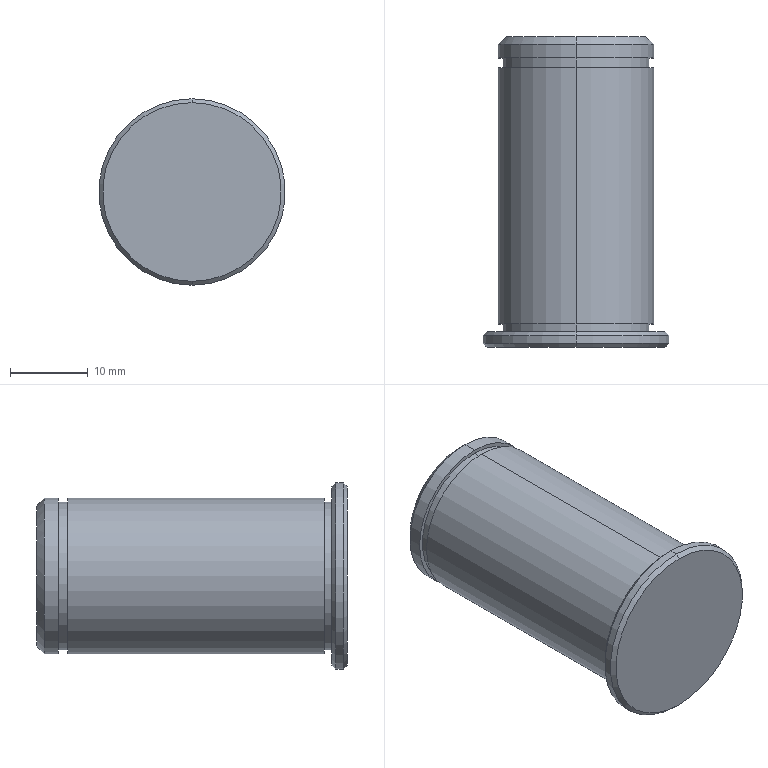Part | SolidWorks | features Revolution 1 | 1 solid | 22 faces | box 24 x 40 x 24 mm | volume 12725 mm3 | cylinder 10 | cone 6 | plane 6 | commonest cylinder face diameters 19 x4 20 x4 24 x2
STEP:
#1=CARTESIAN_POINT('',(0.,0.,-11.5));
#2=VERTEX_POINT('',#1);
#3=CARTESIAN_POINT('',(0.,0.,11.5));
#4=VERTEX_POINT('',#3);
#5=CARTESIAN_POINT('',(0.,0.,0.));
#6=DIRECTION('',(0.,-1.,0.));
#7=DIRECTION('',(0.,0.,-1.));
#8=AXIS2_PLACEMENT_3D('',#5,#6,#7);
#9=CIRCLE('',#8,11.5);
#10=EDGE_CURVE('',#2,#4,#9,.T.);
#11=ORIENTED_EDGE('',*,*,#10,.F.);
#12=CARTESIAN_POINT('',(0.,0.5,-12.));
#13=VERTEX_POINT('',#12);
#14=CARTESIAN_POINT('',(0.,0.,-11.5));
#15=DIRECTION('',(0.,0.7071,-0.7071));
#16=VECTOR('',#15,1000.);
#17=LINE('',#14,#16);
#18=EDGE_CURVE('',#2,#13,#17,.T.);
#19=ORIENTED_EDGE('',*,*,#18,.T.);
#20=CARTESIAN_POINT('',(0.,0.5,12.));
#21=VERTEX_POINT('',#20);
#22=CARTESIAN_POINT('',(0.,0.5,0.));
#23=DIRECTION('',(0.,-1.,0.));
#24=DIRECTION('',(0.,0.,-1.));
#25=AXIS2_PLACEMENT_3D('',#22,#23,#24);
#26=CIRCLE('',#25,12.);
#27=EDGE_CURVE('',#13,#21,#26,.T.);
#28=ORIENTED_EDGE('',*,*,#27,.T.);
#29=CARTESIAN_POINT('',(0.,0.,11.5));
#30=DIRECTION('',(0.,0.7071,0.7071));
#31=VECTOR('',#30,1000.);
#32=LINE('',#29,#31);
#33=EDGE_CURVE('',#4,#21,#32,.T.);
#34=ORIENTED_EDGE('',*,*,#33,.F.);
#35=EDGE_LOOP('',(#11,#19,#28,#34));
#36=FACE_OUTER_BOUND('',#35,.T.);
#37=CARTESIAN_POINT('',(0.,0.,0.));
#38=DIRECTION('',(0.,1.,0.));
#39=DIRECTION('',(0.,0.,1.));
#40=AXIS2_PLACEMENT_3D('',#37,#38,#39);
#41=CONICAL_SURFACE('',#40,11.5,0.7854);
#42=ADVANCED_FACE('',(#36),#41,.T.);
#43=CARTESIAN_POINT('',(0.,1.5,-12.));
#44=VERTEX_POINT('',#43);
#45=CARTESIAN_POINT('',(0.,1.5,12.));
#46=VERTEX_POINT('',#45);
#47=CARTESIAN_POINT('',(0.,1.5,0.));
#48=DIRECTION('',(0.,-1.,0.));
#49=DIRECTION('',(0.,0.,-1.));
#50=AXIS2_PLACEMENT_3D('',#47,#48,#49);
#51=CIRCLE('',#50,12.);
#52=EDGE_CURVE('',#44,#46,#51,.T.);
#53=ORIENTED_EDGE('',*,*,#52,.T.);
#54=CARTESIAN_POINT('',(0.,-1.467,12.));
#55=DIRECTION('',(0.,-1.,0.));
#56=VECTOR('',#55,1000.);
#57=LINE('',#54,#56);
#58=EDGE_CURVE('',#46,#21,#57,.T.);
#59=ORIENTED_EDGE('',*,*,#58,.T.);
#60=ORIENTED_EDGE('',*,*,#27,.F.);
#61=CARTESIAN_POINT('',(0.,-1.467,-12.));
#62=DIRECTION('',(0.,-1.,0.));
#63=VECTOR('',#62,1000.);
#64=LINE('',#61,#63);
#65=EDGE_CURVE('',#44,#13,#64,.T.);
#66=ORIENTED_EDGE('',*,*,#65,.F.);
#67=EDGE_LOOP('',(#53,#59,#60,#66));
#68=FACE_OUTER_BOUND('',#67,.T.);
#69=CARTESIAN_POINT('',(0.,-1.467,0.));
#70=DIRECTION('',(0.,-1.,0.));
#71=DIRECTION('',(0.,0.,-1.));
#72=AXIS2_PLACEMENT_3D('',#69,#70,#71);
#73=CYLINDRICAL_SURFACE('',#72,12.);
#74=ADVANCED_FACE('',(#68),#73,.T.);
#75=CARTESIAN_POINT('',(0.,2.,-11.5));
#76=VERTEX_POINT('',#75);
#77=CARTESIAN_POINT('',(0.,2.,11.5));
#78=VERTEX_POINT('',#77);
#79=CARTESIAN_POINT('',(0.,2.,0.));
#80=DIRECTION('',(0.,-1.,0.));
#81=DIRECTION('',(0.,0.,-1.));
#82=AXIS2_PLACEMENT_3D('',#79,#80,#81);
#83=CIRCLE('',#82,11.5);
#84=EDGE_CURVE('',#76,#78,#83,.T.);
#85=ORIENTED_EDGE('',*,*,#84,.T.);
#86=CARTESIAN_POINT('',(0.,1.5,12.));
#87=DIRECTION('',(0.,-0.7071,0.7071));
#88=VECTOR('',#87,1000.);
#89=LINE('',#86,#88);
#90=EDGE_CURVE('',#78,#46,#89,.T.);
#91=ORIENTED_EDGE('',*,*,#90,.T.);
#92=ORIENTED_EDGE('',*,*,#52,.F.);
#93=CARTESIAN_POINT('',(0.,1.5,-12.));
#94=DIRECTION('',(0.,-0.7071,-0.7071));
#95=VECTOR('',#94,1000.);
#96=LINE('',#93,#95);
#97=EDGE_CURVE('',#76,#44,#96,.T.);
#98=ORIENTED_EDGE('',*,*,#97,.F.);
#99=EDGE_LOOP('',(#85,#91,#92,#98));
#100=FACE_OUTER_BOUND('',#99,.T.);
#101=CARTESIAN_POINT('',(0.,1.5,0.));
#102=DIRECTION('',(0.,-1.,0.));
#103=DIRECTION('',(0.,0.,-1.));
#104=AXIS2_PLACEMENT_3D('',#101,#102,#103);
#105=CONICAL_SURFACE('',#104,12.,0.7854);
#106=ADVANCED_FACE('',(#100),#105,.T.);
#107=CARTESIAN_POINT('',(0.,3.,-9.5));
#108=VERTEX_POINT('',#107);
#109=CARTESIAN_POINT('',(0.,3.,9.5));
#110=VERTEX_POINT('',#109);
#111=CARTESIAN_POINT('',(0.,3.,0.));
#112=DIRECTION('',(0.,-1.,0.));
#113=DIRECTION('',(0.,0.,-1.));
#114=AXIS2_PLACEMENT_3D('',#111,#112,#113);
#115=CIRCLE('',#114,9.5);
#116=EDGE_CURVE('',#108,#110,#115,.T.);
#117=ORIENTED_EDGE('',*,*,#116,.T.);
#118=CARTESIAN_POINT('',(0.,2.,9.5));
#119=VERTEX_POINT('',#118);
#120=CARTESIAN_POINT('',(0.,-1.467,9.5));
#121=DIRECTION('',(0.,-1.,0.));
#122=VECTOR('',#121,1000.);
#123=LINE('',#120,#122);
#124=EDGE_CURVE('',#110,#119,#123,.T.);
#125=ORIENTED_EDGE('',*,*,#124,.T.);
#126=CARTESIAN_POINT('',(0.,2.,-9.5));
#127=VERTEX_POINT('',#126);
#128=CARTESIAN_POINT('',(0.,2.,0.));
#129=DIRECTION('',(0.,-1.,0.));
#130=DIRECTION('',(0.,0.,-1.));
#131=AXIS2_PLACEMENT_3D('',#128,#129,#130);
#132=CIRCLE('',#131,9.5);
#133=EDGE_CURVE('',#127,#119,#132,.T.);
#134=ORIENTED_EDGE('',*,*,#133,.F.);
#135=CARTESIAN_POINT('',(0.,-1.467,-9.5));
#136=DIRECTION('',(0.,-1.,0.));
#137=VECTOR('',#136,1000.);
#138=LINE('',#135,#137);
#139=EDGE_CURVE('',#108,#127,#138,.T.);
#140=ORIENTED_EDGE('',*,*,#139,.F.);
#141=EDGE_LOOP('',(#117,#125,#134,#140));
#142=FACE_OUTER_BOUND('',#141,.T.);
#143=CARTESIAN_POINT('',(0.,-1.467,0.));
#144=DIRECTION('',(0.,-1.,0.));
#145=DIRECTION('',(0.,0.,-1.));
#146=AXIS2_PLACEMENT_3D('',#143,#144,#145);
#147=CYLINDRICAL_SURFACE('',#146,9.5);
#148=ADVANCED_FACE('',(#142),#147,.T.);
#149=CARTESIAN_POINT('',(0.,36.,-10.));
#150=VERTEX_POINT('',#149);
#151=CARTESIAN_POINT('',(0.,36.,10.));
#152=VERTEX_POINT('',#151);
#153=CARTESIAN_POINT('',(0.,36.,0.));
#154=DIRECTION('',(0.,-1.,0.));
#155=DIRECTION('',(0.,0.,-1.));
#156=AXIS2_PLACEMENT_3D('',#153,#154,#155);
#157=CIRCLE('',#156,10.);
#158=EDGE_CURVE('',#150,#152,#157,.T.);
#159=ORIENTED_EDGE('',*,*,#158,.T.);
#160=CARTESIAN_POINT('',(0.,3.,10.));
#161=VERTEX_POINT('',#160);
#162=CARTESIAN_POINT('',(0.,-1.467,10.));
#163=DIRECTION('',(0.,-1.,0.));
#164=VECTOR('',#163,1000.);
#165=LINE('',#162,#164);
#166=EDGE_CURVE('',#152,#161,#165,.T.);
#167=ORIENTED_EDGE('',*,*,#166,.T.);
#168=CARTESIAN_POINT('',(0.,3.,-10.));
#169=VERTEX_POINT('',#168);
#170=CARTESIAN_POINT('',(0.,3.,0.));
#171=DIRECTION('',(0.,-1.,0.));
#172=DIRECTION('',(0.,0.,-1.));
#173=AXIS2_PLACEMENT_3D('',#170,#171,#172);
#174=CIRCLE('',#173,10.);
#175=EDGE_CURVE('',#169,#161,#174,.T.);
#176=ORIENTED_EDGE('',*,*,#175,.F.);
#177=CARTESIAN_POINT('',(0.,-1.467,-10.));
#178=DIRECTION('',(0.,-1.,0.));
#179=VECTOR('',#178,1000.);
#180=LINE('',#177,#179);
#181=EDGE_CURVE('',#150,#169,#180,.T.);
#182=ORIENTED_EDGE('',*,*,#181,.F.);
#183=EDGE_LOOP('',(#159,#167,#176,#182));
#184=FACE_OUTER_BOUND('',#183,.T.);
#185=CARTESIAN_POINT('',(0.,-1.467,0.));
#186=DIRECTION('',(0.,-1.,0.));
#187=DIRECTION('',(0.,0.,-1.));
#188=AXIS2_PLACEMENT_3D('',#185,#186,#187);
#189=CYLINDRICAL_SURFACE('',#188,10.);
#190=ADVANCED_FACE('',(#184),#189,.T.);
#191=CARTESIAN_POINT('',(0.,37.25,-9.5));
#192=VERTEX_POINT('',#191);
#193=CARTESIAN_POINT('',(0.,37.25,9.5));
#194=VERTEX_POINT('',#193);
#195=CARTESIAN_POINT('',(0.,37.25,0.));
#196=DIRECTION('',(0.,-1.,0.));
#197=DIRECTION('',(0.,0.,-1.));
#198=AXIS2_PLACEMENT_3D('',#195,#196,#197);
#199=CIRCLE('',#198,9.5);
#200=EDGE_CURVE('',#192,#194,#199,.T.);
#201=ORIENTED_EDGE('',*,*,#200,.T.);
#202=CARTESIAN_POINT('',(0.,36.,9.5));
#203=VERTEX_POINT('',#202);
#204=CARTESIAN_POINT('',(0.,-1.467,9.5));
#205=DIRECTION('',(0.,-1.,0.));
#206=VECTOR('',#205,1000.);
#207=LINE('',#204,#206);
#208=EDGE_CURVE('',#194,#203,#207,.T.);
#209=ORIENTED_EDGE('',*,*,#208,.T.);
#210=CARTESIAN_POINT('',(0.,36.,-9.5));
#211=VERTEX_POINT('',#210);
#212=CARTESIAN_POINT('',(0.,36.,0.));
#213=DIRECTION('',(0.,-1.,0.));
#214=DIRECTION('',(0.,0.,-1.));
#215=AXIS2_PLACEMENT_3D('',#212,#213,#214);
#216=CIRCLE('',#215,9.5);
#217=EDGE_CURVE('',#211,#203,#216,.T.);
#218=ORIENTED_EDGE('',*,*,#217,.F.);
#219=CARTESIAN_POINT('',(0.,-1.467,-9.5));
#220=DIRECTION('',(0.,-1.,0.));
#221=VECTOR('',#220,1000.);
#222=LINE('',#219,#221);
#223=EDGE_CURVE('',#192,#211,#222,.T.);
#224=ORIENTED_EDGE('',*,*,#223,.F.);
#225=EDGE_LOOP('',(#201,#209,#218,#224));
#226=FACE_OUTER_BOUND('',#225,.T.);
#227=CARTESIAN_POINT('',(0.,-1.467,0.));
#228=DIRECTION('',(0.,-1.,0.));
#229=DIRECTION('',(0.,0.,-1.));
#230=AXIS2_PLACEMENT_3D('',#227,#228,#229);
#231=CYLINDRICAL_SURFACE('',#230,9.5);
#232=ADVANCED_FACE('',(#226),#231,.T.);
#233=CARTESIAN_POINT('',(0.,39.,-10.));
#234=VERTEX_POINT('',#233);
#235=CARTESIAN_POINT('',(0.,39.,10.));
#236=VERTEX_POINT('',#235);
#237=CARTESIAN_POINT('',(0.,39.,0.));
#238=DIRECTION('',(0.,-1.,0.));
#239=DIRECTION('',(0.,0.,-1.));
#240=AXIS2_PLACEMENT_3D('',#237,#238,#239);
#241=CIRCLE('',#240,10.);
#242=EDGE_CURVE('',#234,#236,#241,.T.);
#243=ORIENTED_EDGE('',*,*,#242,.T.);
#244=CARTESIAN_POINT('',(0.,37.25,10.));
#245=VERTEX_POINT('',#244);
#246=CARTESIAN_POINT('',(0.,-1.467,10.));
#247=DIRECTION('',(0.,-1.,0.));
#248=VECTOR('',#247,1000.);
#249=LINE('',#246,#248);
#250=EDGE_CURVE('',#236,#245,#249,.T.);
#251=ORIENTED_EDGE('',*,*,#250,.T.);
#252=CARTESIAN_POINT('',(0.,37.25,-10.));
#253=VERTEX_POINT('',#252);
#254=CARTESIAN_POINT('',(0.,37.25,0.));
#255=DIRECTION('',(0.,-1.,0.));
#256=DIRECTION('',(0.,0.,-1.));
#257=AXIS2_PLACEMENT_3D('',#254,#255,#256);
#258=CIRCLE('',#257,10.);
#259=EDGE_CURVE('',#253,#245,#258,.T.);
#260=ORIENTED_EDGE('',*,*,#259,.F.);
#261=CARTESIAN_POINT('',(0.,-1.467,-10.));
#262=DIRECTION('',(0.,-1.,0.));
#263=VECTOR('',#262,1000.);
#264=LINE('',#261,#263);
#265=EDGE_CURVE('',#234,#253,#264,.T.);
#266=ORIENTED_EDGE('',*,*,#265,.F.);
#267=EDGE_LOOP('',(#243,#251,#260,#266));
#268=FACE_OUTER_BOUND('',#267,.T.);
#269=CARTESIAN_POINT('',(0.,-1.467,0.));
#270=DIRECTION('',(0.,-1.,0.));
#271=DIRECTION('',(0.,0.,-1.));
#272=AXIS2_PLACEMENT_3D('',#269,#270,#271);
#273=CYLINDRICAL_SURFACE('',#272,10.);
#274=ADVANCED_FACE('',(#268),#273,.T.);
#275=CARTESIAN_POINT('',(0.,40.,-9.));
#276=VERTEX_POINT('',#275);
#277=CARTESIAN_POINT('',(0.,40.,9.));
#278=VERTEX_POINT('',#277);
#279=CARTESIAN_POINT('',(0.,40.,0.));
#280=DIRECTION('',(0.,-1.,0.));
#281=DIRECTION('',(0.,0.,-1.));
#282=AXIS2_PLACEMENT_3D('',#279,#280,#281);
#283=CIRCLE('',#282,9.);
#284=EDGE_CURVE('',#276,#278,#283,.T.);
#285=ORIENTED_EDGE('',*,*,#284,.T.);
#286=CARTESIAN_POINT('',(0.,39.,10.));
#287=DIRECTION('',(0.,-0.7071,0.7071));
#288=VECTOR('',#287,1000.);
#289=LINE('',#286,#288);
#290=EDGE_CURVE('',#278,#236,#289,.T.);
#291=ORIENTED_EDGE('',*,*,#290,.T.);
#292=ORIENTED_EDGE('',*,*,#242,.F.);
#293=CARTESIAN_POINT('',(0.,39.,-10.));
#294=DIRECTION('',(0.,-0.7071,-0.7071));
#295=VECTOR('',#294,1000.);
#296=LINE('',#293,#295);
#297=EDGE_CURVE('',#276,#234,#296,.T.);
#298=ORIENTED_EDGE('',*,*,#297,.F.);
#299=EDGE_LOOP('',(#285,#291,#292,#298));
#300=FACE_OUTER_BOUND('',#299,.T.);
#301=CARTESIAN_POINT('',(0.,39.,0.));
#302=DIRECTION('',(0.,-1.,0.));
#303=DIRECTION('',(0.,0.,-1.));
#304=AXIS2_PLACEMENT_3D('',#301,#302,#303);
#305=CONICAL_SURFACE('',#304,10.,0.7854);
#306=ADVANCED_FACE('',(#300),#305,.T.);
#307=ORIENTED_EDGE('',*,*,#284,.F.);
#308=CARTESIAN_POINT('',(0.,40.,0.));
#309=DIRECTION('',(0.,-1.,0.));
#310=DIRECTION('',(0.,0.,-1.));
#311=AXIS2_PLACEMENT_3D('',#308,#309,#310);
#312=CIRCLE('',#311,9.);
#313=EDGE_CURVE('',#278,#276,#312,.T.);
#314=ORIENTED_EDGE('',*,*,#313,.F.);
#315=EDGE_LOOP('',(#307,#314));
#316=FACE_OUTER_BOUND('',#315,.T.);
#317=CARTESIAN_POINT('',(0.,40.,0.));
#318=DIRECTION('',(0.,1.,0.));
#319=DIRECTION('',(0.,0.,1.));
#320=AXIS2_PLACEMENT_3D('',#317,#318,#319);
#321=PLANE('',#320);
#322=ADVANCED_FACE('',(#316),#321,.T.);
#323=ORIENTED_EDGE('',*,*,#290,.F.);
#324=ORIENTED_EDGE('',*,*,#313,.T.);
#325=ORIENTED_EDGE('',*,*,#297,.T.);
#326=CARTESIAN_POINT('',(0.,39.,0.));
#327=DIRECTION('',(0.,-1.,0.));
#328=DIRECTION('',(0.,0.,-1.));
#329=AXIS2_PLACEMENT_3D('',#326,#327,#328);
#330=CIRCLE('',#329,10.);
#331=EDGE_CURVE('',#236,#234,#330,.T.);
#332=ORIENTED_EDGE('',*,*,#331,.F.);
#333=EDGE_LOOP('',(#323,#324,#325,#332));
#334=FACE_OUTER_BOUND('',#333,.T.);
#335=CARTESIAN_POINT('',(0.,39.,0.));
#336=DIRECTION('',(0.,-1.,0.));
#337=DIRECTION('',(0.,0.,-1.));
#338=AXIS2_PLACEMENT_3D('',#335,#336,#337);
#339=CONICAL_SURFACE('',#338,10.,0.7854);
#340=ADVANCED_FACE('',(#334),#339,.T.);
#341=ORIENTED_EDGE('',*,*,#250,.F.);
#342=ORIENTED_EDGE('',*,*,#331,.T.);
#343=ORIENTED_EDGE('',*,*,#265,.T.);
#344=CARTESIAN_POINT('',(0.,37.25,0.));
#345=DIRECTION('',(0.,-1.,0.));
#346=DIRECTION('',(0.,0.,-1.));
#347=AXIS2_PLACEMENT_3D('',#344,#345,#346);
#348=CIRCLE('',#347,10.);
#349=EDGE_CURVE('',#245,#253,#348,.T.);
#350=ORIENTED_EDGE('',*,*,#349,.F.);
#351=EDGE_LOOP('',(#341,#342,#343,#350));
#352=FACE_OUTER_BOUND('',#351,.T.);
#353=CARTESIAN_POINT('',(0.,-1.467,0.));
#354=DIRECTION('',(0.,-1.,0.));
#355=DIRECTION('',(0.,0.,-1.));
#356=AXIS2_PLACEMENT_3D('',#353,#354,#355);
#357=CYLINDRICAL_SURFACE('',#356,10.);
#358=ADVANCED_FACE('',(#352),#357,.T.);
#359=ORIENTED_EDGE('',*,*,#259,.T.);
#360=ORIENTED_EDGE('',*,*,#349,.T.);
#361=EDGE_LOOP('',(#359,#360));
#362=FACE_OUTER_BOUND('',#361,.T.);
#363=ORIENTED_EDGE('',*,*,#200,.F.);
#364=CARTESIAN_POINT('',(0.,37.25,0.));
#365=DIRECTION('',(0.,-1.,0.));
#366=DIRECTION('',(0.,0.,-1.));
#367=AXIS2_PLACEMENT_3D('',#364,#365,#366);
#368=CIRCLE('',#367,9.5);
#369=EDGE_CURVE('',#194,#192,#368,.T.);
#370=ORIENTED_EDGE('',*,*,#369,.F.);
#371=EDGE_LOOP('',(#363,#370));
#372=FACE_BOUND('',#371,.T.);
#373=CARTESIAN_POINT('',(10.,37.25,0.));
#374=DIRECTION('',(0.,-1.,0.));
#375=DIRECTION('',(0.,0.,-1.));
#376=AXIS2_PLACEMENT_3D('',#373,#374,#375);
#377=PLANE('',#376);
#378=ADVANCED_FACE('',(#362,#372),#377,.T.);
#379=ORIENTED_EDGE('',*,*,#208,.F.);
#380=ORIENTED_EDGE('',*,*,#369,.T.);
#381=ORIENTED_EDGE('',*,*,#223,.T.);
#382=CARTESIAN_POINT('',(0.,36.,0.));
#383=DIRECTION('',(0.,-1.,0.));
#384=DIRECTION('',(0.,0.,-1.));
#385=AXIS2_PLACEMENT_3D('',#382,#383,#384);
#386=CIRCLE('',#385,9.5);
#387=EDGE_CURVE('',#203,#211,#386,.T.);
#388=ORIENTED_EDGE('',*,*,#387,.F.);
#389=EDGE_LOOP('',(#379,#380,#381,#388));
#390=FACE_OUTER_BOUND('',#389,.T.);
#391=CARTESIAN_POINT('',(0.,-1.467,0.));
#392=DIRECTION('',(0.,-1.,0.));
#393=DIRECTION('',(0.,0.,-1.));
#394=AXIS2_PLACEMENT_3D('',#391,#392,#393);
#395=CYLINDRICAL_SURFACE('',#394,9.5);
#396=ADVANCED_FACE('',(#390),#395,.T.);
#397=ORIENTED_EDGE('',*,*,#217,.T.);
#398=ORIENTED_EDGE('',*,*,#387,.T.);
#399=EDGE_LOOP('',(#397,#398));
#400=FACE_BOUND('',#399,.T.);
#401=ORIENTED_EDGE('',*,*,#158,.F.);
#402=CARTESIAN_POINT('',(0.,36.,0.));
#403=DIRECTION('',(0.,-1.,0.));
#404=DIRECTION('',(0.,0.,-1.));
#405=AXIS2_PLACEMENT_3D('',#402,#403,#404);
#406=CIRCLE('',#405,10.);
#407=EDGE_CURVE('',#152,#150,#406,.T.);
#408=ORIENTED_EDGE('',*,*,#407,.F.);
#409=EDGE_LOOP('',(#401,#408));
#410=FACE_OUTER_BOUND('',#409,.T.);
#411=CARTESIAN_POINT('',(9.5,36.,0.));
#412=DIRECTION('',(0.,1.,0.));
#413=DIRECTION('',(0.,0.,1.));
#414=AXIS2_PLACEMENT_3D('',#411,#412,#413);
#415=PLANE('',#414);
#416=ADVANCED_FACE('',(#400,#410),#415,.T.);
#417=ORIENTED_EDGE('',*,*,#166,.F.);
#418=ORIENTED_EDGE('',*,*,#407,.T.);
#419=ORIENTED_EDGE('',*,*,#181,.T.);
#420=CARTESIAN_POINT('',(0.,3.,0.));
#421=DIRECTION('',(0.,-1.,0.));
#422=DIRECTION('',(0.,0.,-1.));
#423=AXIS2_PLACEMENT_3D('',#420,#421,#422);
#424=CIRCLE('',#423,10.);
#425=EDGE_CURVE('',#161,#169,#424,.T.);
#426=ORIENTED_EDGE('',*,*,#425,.F.);
#427=EDGE_LOOP('',(#417,#418,#419,#426));
#428=FACE_OUTER_BOUND('',#427,.T.);
#429=CARTESIAN_POINT('',(0.,-1.467,0.));
#430=DIRECTION('',(0.,-1.,0.));
#431=DIRECTION('',(0.,0.,-1.));
#432=AXIS2_PLACEMENT_3D('',#429,#430,#431);
#433=CYLINDRICAL_SURFACE('',#432,10.);
#434=ADVANCED_FACE('',(#428),#433,.T.);
#435=ORIENTED_EDGE('',*,*,#175,.T.);
#436=ORIENTED_EDGE('',*,*,#425,.T.);
#437=EDGE_LOOP('',(#435,#436));
#438=FACE_OUTER_BOUND('',#437,.T.);
#439=ORIENTED_EDGE('',*,*,#116,.F.);
#440=CARTESIAN_POINT('',(0.,3.,0.));
#441=DIRECTION('',(0.,-1.,0.));
#442=DIRECTION('',(0.,0.,-1.));
#443=AXIS2_PLACEMENT_3D('',#440,#441,#442);
#444=CIRCLE('',#443,9.5);
#445=EDGE_CURVE('',#110,#108,#444,.T.);
#446=ORIENTED_EDGE('',*,*,#445,.F.);
#447=EDGE_LOOP('',(#439,#446));
#448=FACE_BOUND('',#447,.T.);
#449=CARTESIAN_POINT('',(9.5,3.,0.));
#450=DIRECTION('',(0.,-1.,0.));
#451=DIRECTION('',(0.,0.,-1.));
#452=AXIS2_PLACEMENT_3D('',#449,#450,#451);
#453=PLANE('',#452);
#454=ADVANCED_FACE('',(#438,#448),#453,.T.);
#455=ORIENTED_EDGE('',*,*,#124,.F.);
#456=ORIENTED_EDGE('',*,*,#445,.T.);
#457=ORIENTED_EDGE('',*,*,#139,.T.);
#458=CARTESIAN_POINT('',(0.,2.,0.));
#459=DIRECTION('',(0.,-1.,0.));
#460=DIRECTION('',(0.,0.,-1.));
#461=AXIS2_PLACEMENT_3D('',#458,#459,#460);
#462=CIRCLE('',#461,9.5);
#463=EDGE_CURVE('',#119,#127,#462,.T.);
#464=ORIENTED_EDGE('',*,*,#463,.F.);
#465=EDGE_LOOP('',(#455,#456,#457,#464));
#466=FACE_OUTER_BOUND('',#465,.T.);
#467=CARTESIAN_POINT('',(0.,-1.467,0.));
#468=DIRECTION('',(0.,-1.,0.));
#469=DIRECTION('',(0.,0.,-1.));
#470=AXIS2_PLACEMENT_3D('',#467,#468,#469);
#471=CYLINDRICAL_SURFACE('',#470,9.5);
#472=ADVANCED_FACE('',(#466),#471,.T.);
#473=ORIENTED_EDGE('',*,*,#133,.T.);
#474=ORIENTED_EDGE('',*,*,#463,.T.);
#475=EDGE_LOOP('',(#473,#474));
#476=FACE_BOUND('',#475,.T.);
#477=ORIENTED_EDGE('',*,*,#84,.F.);
#478=CARTESIAN_POINT('',(0.,2.,0.));
#479=DIRECTION('',(0.,-1.,0.));
#480=DIRECTION('',(0.,0.,-1.));
#481=AXIS2_PLACEMENT_3D('',#478,#479,#480);
#482=CIRCLE('',#481,11.5);
#483=EDGE_CURVE('',#78,#76,#482,.T.);
#484=ORIENTED_EDGE('',*,*,#483,.F.);
#485=EDGE_LOOP('',(#477,#484));
#486=FACE_OUTER_BOUND('',#485,.T.);
#487=CARTESIAN_POINT('',(11.5,2.,0.));
#488=DIRECTION('',(0.,1.,0.));
#489=DIRECTION('',(0.,0.,1.));
#490=AXIS2_PLACEMENT_3D('',#487,#488,#489);
#491=PLANE('',#490);
#492=ADVANCED_FACE('',(#476,#486),#491,.T.);
#493=ORIENTED_EDGE('',*,*,#90,.F.);
#494=ORIENTED_EDGE('',*,*,#483,.T.);
#495=ORIENTED_EDGE('',*,*,#97,.T.);
#496=CARTESIAN_POINT('',(0.,1.5,0.));
#497=DIRECTION('',(0.,-1.,0.));
#498=DIRECTION('',(0.,0.,-1.));
#499=AXIS2_PLACEMENT_3D('',#496,#497,#498);
#500=CIRCLE('',#499,12.);
#501=EDGE_CURVE('',#46,#44,#500,.T.);
#502=ORIENTED_EDGE('',*,*,#501,.F.);
#503=EDGE_LOOP('',(#493,#494,#495,#502));
#504=FACE_OUTER_BOUND('',#503,.T.);
#505=CARTESIAN_POINT('',(0.,1.5,0.));
#506=DIRECTION('',(0.,-1.,0.));
#507=DIRECTION('',(0.,0.,-1.));
#508=AXIS2_PLACEMENT_3D('',#505,#506,#507);
#509=CONICAL_SURFACE('',#508,12.,0.7854);
#510=ADVANCED_FACE('',(#504),#509,.T.);
#511=ORIENTED_EDGE('',*,*,#58,.F.);
#512=ORIENTED_EDGE('',*,*,#501,.T.);
#513=ORIENTED_EDGE('',*,*,#65,.T.);
#514=CARTESIAN_POINT('',(0.,0.5,0.));
#515=DIRECTION('',(0.,-1.,0.));
#516=DIRECTION('',(0.,0.,-1.));
#517=AXIS2_PLACEMENT_3D('',#514,#515,#516);
#518=CIRCLE('',#517,12.);
#519=EDGE_CURVE('',#21,#13,#518,.T.);
#520=ORIENTED_EDGE('',*,*,#519,.F.);
#521=EDGE_LOOP('',(#511,#512,#513,#520));
#522=FACE_OUTER_BOUND('',#521,.T.);
#523=CARTESIAN_POINT('',(0.,-1.467,0.));
#524=DIRECTION('',(0.,-1.,0.));
#525=DIRECTION('',(0.,0.,-1.));
#526=AXIS2_PLACEMENT_3D('',#523,#524,#525);
#527=CYLINDRICAL_SURFACE('',#526,12.);
#528=ADVANCED_FACE('',(#522),#527,.T.);
#529=ORIENTED_EDGE('',*,*,#18,.F.);
#530=CARTESIAN_POINT('',(0.,0.,0.));
#531=DIRECTION('',(0.,-1.,0.));
#532=DIRECTION('',(0.,0.,-1.));
#533=AXIS2_PLACEMENT_3D('',#530,#531,#532);
#534=CIRCLE('',#533,11.5);
#535=EDGE_CURVE('',#4,#2,#534,.T.);
#536=ORIENTED_EDGE('',*,*,#535,.F.);
#537=ORIENTED_EDGE('',*,*,#33,.T.);
#538=ORIENTED_EDGE('',*,*,#519,.T.);
#539=EDGE_LOOP('',(#529,#536,#537,#538));
#540=FACE_OUTER_BOUND('',#539,.T.);
#541=CARTESIAN_POINT('',(0.,0.,0.));
#542=DIRECTION('',(0.,1.,0.));
#543=DIRECTION('',(0.,0.,1.));
#544=AXIS2_PLACEMENT_3D('',#541,#542,#543);
#545=CONICAL_SURFACE('',#544,11.5,0.7854);
#546=ADVANCED_FACE('',(#540),#545,.T.);
#547=ORIENTED_EDGE('',*,*,#535,.T.);
#548=ORIENTED_EDGE('',*,*,#10,.T.);
#549=EDGE_LOOP('',(#547,#548));
#550=FACE_OUTER_BOUND('',#549,.T.);
#551=CARTESIAN_POINT('',(0.,0.,0.));
#552=DIRECTION('',(0.,-1.,0.));
#553=DIRECTION('',(0.,0.,-1.));
#554=AXIS2_PLACEMENT_3D('',#551,#552,#553);
#555=PLANE('',#554);
#556=ADVANCED_FACE('',(#550),#555,.T.);
#557=CLOSED_SHELL('',(#42,#74,#106,#148,#190,#232,#274,#306,#322,#340,#358,#378,#396,#416,#434,#454,#472,#492,#510,#528,#546,#556));
#558=MANIFOLD_SOLID_BREP('',#557);
#559=CARTESIAN_POINT('',(0.,0.,0.));
#560=DIRECTION('',(0.,0.,1.));
#561=DIRECTION('',(1.,0.,0.));
#562=AXIS2_PLACEMENT_3D('',#559,#560,#561);
#563=(LENGTH_UNIT()NAMED_UNIT(*)SI_UNIT(.MILLI.,.METRE.));
#564=UNCERTAINTY_MEASURE_WITH_UNIT(LENGTH_MEASURE(0.00001),#563,'','');
#565=(NAMED_UNIT(*)PLANE_ANGLE_UNIT()SI_UNIT($,.RADIAN.));
#566=(NAMED_UNIT(*)SI_UNIT($,.STERADIAN.)SOLID_ANGLE_UNIT());
#567=(GEOMETRIC_REPRESENTATION_CONTEXT(3)GLOBAL_UNCERTAINTY_ASSIGNED_CONTEXT((#564))GLOBAL_UNIT_ASSIGNED_CONTEXT((#563,#565,#566))REPRESENTATION_CONTEXT('',''));
#568=ADVANCED_BREP_SHAPE_REPRESENTATION('',(#558,#562),#567);